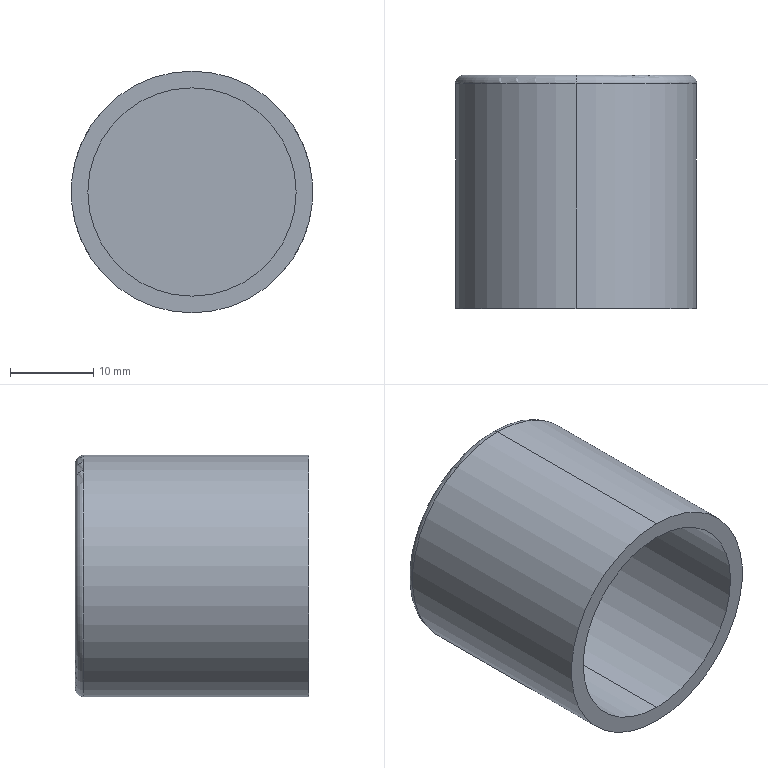Part | SolidWorks | features Fillet 1, Revolution 1 | 1 solid | 9 faces | box 29 x 28 x 29 mm | volume 5713 mm3 | cylinder 4 | plane 3 | torus 2 | commonest cylinder face diameters 25 x2 29 x2
STEP:
#1=CARTESIAN_POINT('',(0.,-1.,-14.5));
#2=VERTEX_POINT('',#1);
#3=CARTESIAN_POINT('',(0.,-1.,14.5));
#4=VERTEX_POINT('',#3);
#5=CARTESIAN_POINT('',(0.,-1.,0.));
#6=DIRECTION('',(0.,-1.,0.));
#7=DIRECTION('',(0.,0.,1.));
#8=AXIS2_PLACEMENT_3D('',#5,#6,#7);
#9=CIRCLE('',#8,14.5);
#10=EDGE_CURVE('',#2,#4,#9,.T.);
#11=ORIENTED_EDGE('',*,*,#10,.F.);
#12=CARTESIAN_POINT('',(0.,0.,-13.5));
#13=VERTEX_POINT('',#12);
#14=CARTESIAN_POINT('',(0.,-1.,-13.5));
#15=DIRECTION('',(1.,0.,0.));
#16=DIRECTION('',(0.,0.,-1.));
#17=AXIS2_PLACEMENT_3D('',#14,#15,#16);
#18=CIRCLE('',#17,1.);
#19=EDGE_CURVE('',#2,#13,#18,.T.);
#20=ORIENTED_EDGE('',*,*,#19,.T.);
#21=CARTESIAN_POINT('',(0.,0.,13.5));
#22=VERTEX_POINT('',#21);
#23=CARTESIAN_POINT('',(0.,0.,0.));
#24=DIRECTION('',(0.,1.,0.));
#25=DIRECTION('',(0.,0.,1.));
#26=AXIS2_PLACEMENT_3D('',#23,#24,#25);
#27=CIRCLE('',#26,13.5);
#28=EDGE_CURVE('',#22,#13,#27,.T.);
#29=ORIENTED_EDGE('',*,*,#28,.F.);
#30=CARTESIAN_POINT('',(0.,-1.,13.5));
#31=DIRECTION('',(-1.,0.,0.));
#32=DIRECTION('',(0.,0.,1.));
#33=AXIS2_PLACEMENT_3D('',#30,#31,#32);
#34=CIRCLE('',#33,1.);
#35=EDGE_CURVE('',#4,#22,#34,.T.);
#36=ORIENTED_EDGE('',*,*,#35,.F.);
#37=EDGE_LOOP('',(#11,#20,#29,#36));
#38=FACE_OUTER_BOUND('',#37,.T.);
#39=CARTESIAN_POINT('',(0.,-1.,0.));
#40=DIRECTION('',(0.,1.,0.));
#41=DIRECTION('',(0.,0.,1.));
#42=AXIS2_PLACEMENT_3D('',#39,#40,#41);
#43=TOROIDAL_SURFACE('',#42,13.5,1.);
#44=ADVANCED_FACE('',(#38),#43,.T.);
#45=CARTESIAN_POINT('',(0.,-2.,12.5));
#46=VERTEX_POINT('',#45);
#47=CARTESIAN_POINT('',(0.,-2.,-12.5));
#48=VERTEX_POINT('',#47);
#49=CARTESIAN_POINT('',(0.,-2.,0.));
#50=DIRECTION('',(0.,-1.,0.));
#51=DIRECTION('',(0.,0.,-1.));
#52=AXIS2_PLACEMENT_3D('',#49,#50,#51);
#53=CIRCLE('',#52,12.5);
#54=EDGE_CURVE('',#46,#48,#53,.T.);
#55=ORIENTED_EDGE('',*,*,#54,.F.);
#56=CARTESIAN_POINT('',(0.,-28.,12.5));
#57=VERTEX_POINT('',#56);
#58=CARTESIAN_POINT('',(0.,-2.,12.5));
#59=DIRECTION('',(0.,-1.,0.));
#60=VECTOR('',#59,1000.);
#61=LINE('',#58,#60);
#62=EDGE_CURVE('',#46,#57,#61,.T.);
#63=ORIENTED_EDGE('',*,*,#62,.T.);
#64=CARTESIAN_POINT('',(0.,-28.,-12.5));
#65=VERTEX_POINT('',#64);
#66=CARTESIAN_POINT('',(0.,-28.,0.));
#67=DIRECTION('',(0.,-1.,0.));
#68=DIRECTION('',(0.,0.,-1.));
#69=AXIS2_PLACEMENT_3D('',#66,#67,#68);
#70=CIRCLE('',#69,12.5);
#71=EDGE_CURVE('',#57,#65,#70,.T.);
#72=ORIENTED_EDGE('',*,*,#71,.T.);
#73=CARTESIAN_POINT('',(0.,-2.,-12.5));
#74=DIRECTION('',(0.,-1.,0.));
#75=VECTOR('',#74,1000.);
#76=LINE('',#73,#75);
#77=EDGE_CURVE('',#48,#65,#76,.T.);
#78=ORIENTED_EDGE('',*,*,#77,.F.);
#79=EDGE_LOOP('',(#55,#63,#72,#78));
#80=FACE_OUTER_BOUND('',#79,.T.);
#81=CARTESIAN_POINT('',(0.,-2.,0.));
#82=DIRECTION('',(0.,-1.,0.));
#83=DIRECTION('',(0.,0.,-1.));
#84=AXIS2_PLACEMENT_3D('',#81,#82,#83);
#85=CYLINDRICAL_SURFACE('',#84,12.5);
#86=ADVANCED_FACE('',(#80),#85,.F.);
#87=ORIENTED_EDGE('',*,*,#10,.T.);
#88=CARTESIAN_POINT('',(0.,-28.,14.5));
#89=VERTEX_POINT('',#88);
#90=CARTESIAN_POINT('',(0.,-2.,14.5));
#91=DIRECTION('',(0.,-1.,0.));
#92=VECTOR('',#91,1000.);
#93=LINE('',#90,#92);
#94=EDGE_CURVE('',#4,#89,#93,.T.);
#95=ORIENTED_EDGE('',*,*,#94,.T.);
#96=CARTESIAN_POINT('',(0.,-28.,-14.5));
#97=VERTEX_POINT('',#96);
#98=CARTESIAN_POINT('',(0.,-28.,0.));
#99=DIRECTION('',(0.,-1.,0.));
#100=DIRECTION('',(0.,0.,-1.));
#101=AXIS2_PLACEMENT_3D('',#98,#99,#100);
#102=CIRCLE('',#101,14.5);
#103=EDGE_CURVE('',#97,#89,#102,.T.);
#104=ORIENTED_EDGE('',*,*,#103,.F.);
#105=CARTESIAN_POINT('',(0.,-2.,-14.5));
#106=DIRECTION('',(0.,-1.,0.));
#107=VECTOR('',#106,1000.);
#108=LINE('',#105,#107);
#109=EDGE_CURVE('',#2,#97,#108,.T.);
#110=ORIENTED_EDGE('',*,*,#109,.F.);
#111=EDGE_LOOP('',(#87,#95,#104,#110));
#112=FACE_OUTER_BOUND('',#111,.T.);
#113=CARTESIAN_POINT('',(0.,-2.,0.));
#114=DIRECTION('',(0.,-1.,0.));
#115=DIRECTION('',(0.,0.,-1.));
#116=AXIS2_PLACEMENT_3D('',#113,#114,#115);
#117=CYLINDRICAL_SURFACE('',#116,14.5);
#118=ADVANCED_FACE('',(#112),#117,.T.);
#119=CARTESIAN_POINT('',(0.,-2.,0.));
#120=DIRECTION('',(0.,-1.,0.));
#121=DIRECTION('',(0.,0.,-1.));
#122=AXIS2_PLACEMENT_3D('',#119,#120,#121);
#123=CIRCLE('',#122,12.5);
#124=EDGE_CURVE('',#48,#46,#123,.T.);
#125=ORIENTED_EDGE('',*,*,#124,.T.);
#126=ORIENTED_EDGE('',*,*,#54,.T.);
#127=EDGE_LOOP('',(#125,#126));
#128=FACE_OUTER_BOUND('',#127,.T.);
#129=CARTESIAN_POINT('',(14.5,-2.,0.));
#130=DIRECTION('',(0.,1.,0.));
#131=DIRECTION('',(0.,0.,1.));
#132=AXIS2_PLACEMENT_3D('',#129,#130,#131);
#133=PLANE('',#132);
#134=ADVANCED_FACE('',(#128),#133,.F.);
#135=ORIENTED_EDGE('',*,*,#103,.T.);
#136=CARTESIAN_POINT('',(0.,-28.,0.));
#137=DIRECTION('',(0.,-1.,0.));
#138=DIRECTION('',(0.,0.,-1.));
#139=AXIS2_PLACEMENT_3D('',#136,#137,#138);
#140=CIRCLE('',#139,14.5);
#141=EDGE_CURVE('',#89,#97,#140,.T.);
#142=ORIENTED_EDGE('',*,*,#141,.T.);
#143=EDGE_LOOP('',(#135,#142));
#144=FACE_OUTER_BOUND('',#143,.T.);
#145=CARTESIAN_POINT('',(0.,-28.,0.));
#146=DIRECTION('',(0.,-1.,0.));
#147=DIRECTION('',(0.,0.,-1.));
#148=AXIS2_PLACEMENT_3D('',#145,#146,#147);
#149=CIRCLE('',#148,12.5);
#150=EDGE_CURVE('',#65,#57,#149,.T.);
#151=ORIENTED_EDGE('',*,*,#150,.F.);
#152=ORIENTED_EDGE('',*,*,#71,.F.);
#153=EDGE_LOOP('',(#151,#152));
#154=FACE_BOUND('',#153,.T.);
#155=CARTESIAN_POINT('',(0.,-28.,0.));
#156=DIRECTION('',(0.,-1.,0.));
#157=DIRECTION('',(0.,0.,-1.));
#158=AXIS2_PLACEMENT_3D('',#155,#156,#157);
#159=PLANE('',#158);
#160=ADVANCED_FACE('',(#144,#154),#159,.T.);
#161=ORIENTED_EDGE('',*,*,#94,.F.);
#162=CARTESIAN_POINT('',(0.,-1.,0.));
#163=DIRECTION('',(0.,-1.,0.));
#164=DIRECTION('',(0.,0.,1.));
#165=AXIS2_PLACEMENT_3D('',#162,#163,#164);
#166=CIRCLE('',#165,14.5);
#167=EDGE_CURVE('',#4,#2,#166,.T.);
#168=ORIENTED_EDGE('',*,*,#167,.T.);
#169=ORIENTED_EDGE('',*,*,#109,.T.);
#170=ORIENTED_EDGE('',*,*,#141,.F.);
#171=EDGE_LOOP('',(#161,#168,#169,#170));
#172=FACE_OUTER_BOUND('',#171,.T.);
#173=CARTESIAN_POINT('',(0.,-2.,0.));
#174=DIRECTION('',(0.,-1.,0.));
#175=DIRECTION('',(0.,0.,-1.));
#176=AXIS2_PLACEMENT_3D('',#173,#174,#175);
#177=CYLINDRICAL_SURFACE('',#176,14.5);
#178=ADVANCED_FACE('',(#172),#177,.T.);
#179=ORIENTED_EDGE('',*,*,#62,.F.);
#180=ORIENTED_EDGE('',*,*,#124,.F.);
#181=ORIENTED_EDGE('',*,*,#77,.T.);
#182=ORIENTED_EDGE('',*,*,#150,.T.);
#183=EDGE_LOOP('',(#179,#180,#181,#182));
#184=FACE_OUTER_BOUND('',#183,.T.);
#185=CARTESIAN_POINT('',(0.,-2.,0.));
#186=DIRECTION('',(0.,-1.,0.));
#187=DIRECTION('',(0.,0.,-1.));
#188=AXIS2_PLACEMENT_3D('',#185,#186,#187);
#189=CYLINDRICAL_SURFACE('',#188,12.5);
#190=ADVANCED_FACE('',(#184),#189,.F.);
#191=ORIENTED_EDGE('',*,*,#28,.T.);
#192=CARTESIAN_POINT('',(0.,0.,0.));
#193=DIRECTION('',(0.,1.,0.));
#194=DIRECTION('',(0.,0.,1.));
#195=AXIS2_PLACEMENT_3D('',#192,#193,#194);
#196=CIRCLE('',#195,13.5);
#197=EDGE_CURVE('',#13,#22,#196,.T.);
#198=ORIENTED_EDGE('',*,*,#197,.T.);
#199=EDGE_LOOP('',(#191,#198));
#200=FACE_OUTER_BOUND('',#199,.T.);
#201=CARTESIAN_POINT('',(14.5,0.,0.));
#202=DIRECTION('',(0.,1.,0.));
#203=DIRECTION('',(0.,0.,1.));
#204=AXIS2_PLACEMENT_3D('',#201,#202,#203);
#205=PLANE('',#204);
#206=ADVANCED_FACE('',(#200),#205,.T.);
#207=ORIENTED_EDGE('',*,*,#19,.F.);
#208=ORIENTED_EDGE('',*,*,#167,.F.);
#209=ORIENTED_EDGE('',*,*,#35,.T.);
#210=ORIENTED_EDGE('',*,*,#197,.F.);
#211=EDGE_LOOP('',(#207,#208,#209,#210));
#212=FACE_OUTER_BOUND('',#211,.T.);
#213=CARTESIAN_POINT('',(0.,-1.,0.));
#214=DIRECTION('',(0.,1.,0.));
#215=DIRECTION('',(0.,0.,1.));
#216=AXIS2_PLACEMENT_3D('',#213,#214,#215);
#217=TOROIDAL_SURFACE('',#216,13.5,1.);
#218=ADVANCED_FACE('',(#212),#217,.T.);
#219=CLOSED_SHELL('',(#44,#86,#118,#134,#160,#178,#190,#206,#218));
#220=MANIFOLD_SOLID_BREP('',#219);
#221=CARTESIAN_POINT('',(0.,0.,0.));
#222=DIRECTION('',(0.,0.,1.));
#223=DIRECTION('',(1.,0.,0.));
#224=AXIS2_PLACEMENT_3D('',#221,#222,#223);
#225=(LENGTH_UNIT()NAMED_UNIT(*)SI_UNIT(.MILLI.,.METRE.));
#226=UNCERTAINTY_MEASURE_WITH_UNIT(LENGTH_MEASURE(0.00001),#225,'','');
#227=(NAMED_UNIT(*)PLANE_ANGLE_UNIT()SI_UNIT($,.RADIAN.));
#228=(NAMED_UNIT(*)SI_UNIT($,.STERADIAN.)SOLID_ANGLE_UNIT());
#229=(GEOMETRIC_REPRESENTATION_CONTEXT(3)GLOBAL_UNCERTAINTY_ASSIGNED_CONTEXT((#226))GLOBAL_UNIT_ASSIGNED_CONTEXT((#225,#227,#228))REPRESENTATION_CONTEXT('',''));
#230=ADVANCED_BREP_SHAPE_REPRESENTATION('',(#220,#224),#229);